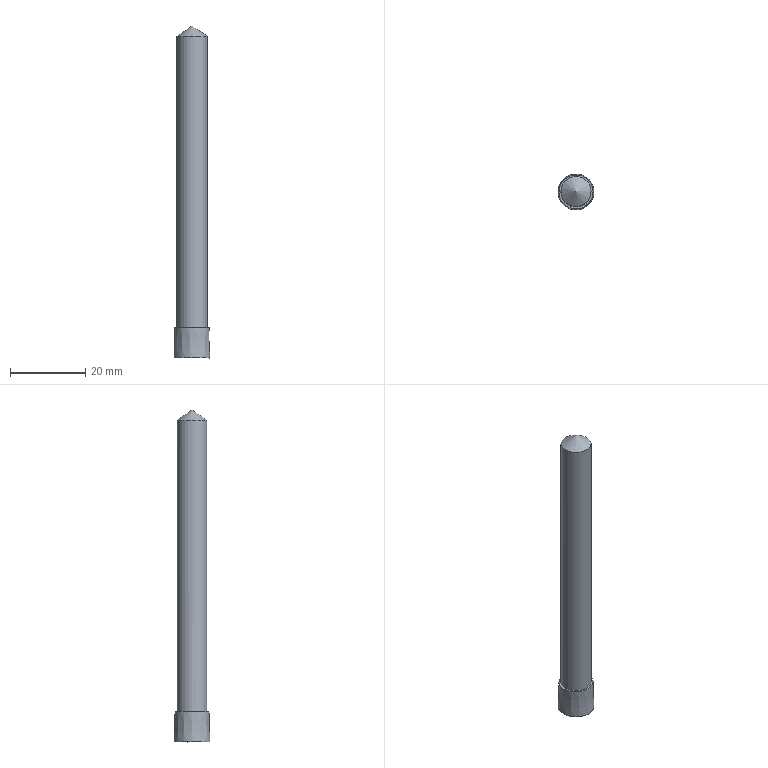Part | STEP file | 车灯-后视镜_id102_x_t | 1 solid | 5 faces | box 9.556 x 9.556 x 88.278 mm | volume 4490 mm3 | plane 2 | cone 2 | cylinder 1 | commonest cylinder face diameters 8 x1
STEP:
#1=CARTESIAN_POINT('',(-132.359,14.875,-27.286));
#2=VERTEX_POINT('',#1);
#3=CARTESIAN_POINT('',(-128.486,15.874,-27.286));
#4=DIRECTION('',(0.,0.,-1.));
#5=DIRECTION('',(-0.9683,-0.2497,0.));
#6=AXIS2_PLACEMENT_3D('',#3,#4,#5);
#7=CIRCLE('',#6,4.);
#8=EDGE_CURVE('',#2,#2,#7,.T.);
#9=ORIENTED_EDGE('',*,*,#8,.T.);
#10=EDGE_LOOP('',(#9));
#11=FACE_BOUND('',#10,.T.);
#12=CARTESIAN_POINT('',(-124.095,17.006,-27.286));
#13=VERTEX_POINT('',#12);
#14=CARTESIAN_POINT('',(-128.486,15.874,-27.286));
#15=DIRECTION('',(0.,0.,1.));
#16=DIRECTION('',(0.9683,0.2497,0.));
#17=AXIS2_PLACEMENT_3D('',#14,#15,#16);
#18=CIRCLE('',#17,4.535);
#19=EDGE_CURVE('',#13,#13,#18,.T.);
#20=ORIENTED_EDGE('',*,*,#19,.T.);
#21=EDGE_LOOP('',(#20));
#22=FACE_BOUND('',#21,.T.);
#23=CARTESIAN_POINT('',(-128.486,15.874,-27.286));
#24=DIRECTION('',(0.,0.,1.));
#25=DIRECTION('',(-0.9683,-0.2497,0.));
#26=AXIS2_PLACEMENT_3D('',#23,#24,#25);
#27=PLANE('',#26);
#28=ADVANCED_FACE('',(#11,#22),#27,.T.);
#29=CARTESIAN_POINT('',(-123.708,15.874,-35.286));
#30=VERTEX_POINT('',#29);
#31=CARTESIAN_POINT('',(-128.486,15.874,-35.286));
#32=DIRECTION('',(0.,0.,-1.));
#33=DIRECTION('',(1.,0.,0.));
#34=AXIS2_PLACEMENT_3D('',#31,#32,#33);
#35=CIRCLE('',#34,4.778);
#36=EDGE_CURVE('',#30,#30,#35,.T.);
#37=ORIENTED_EDGE('',*,*,#36,.F.);
#38=EDGE_LOOP('',(#37));
#39=FACE_BOUND('',#38,.T.);
#40=ORIENTED_EDGE('',*,*,#19,.F.);
#41=EDGE_LOOP('',(#40));
#42=FACE_BOUND('',#41,.T.);
#43=CARTESIAN_POINT('',(-128.486,15.874,-27.286));
#44=DIRECTION('',(0.,0.,-1.));
#45=DIRECTION('',(0.9683,0.2497,0.));
#46=AXIS2_PLACEMENT_3D('',#43,#44,#45);
#47=CONICAL_SURFACE('',#46,4.535,1.738);
#48=ADVANCED_FACE('',(#39,#42),#47,.T.);
#49=ORIENTED_EDGE('',*,*,#8,.F.);
#50=EDGE_LOOP('',(#49));
#51=FACE_BOUND('',#50,.T.);
#52=CARTESIAN_POINT('',(-132.486,15.874,50.294));
#53=VERTEX_POINT('',#52);
#54=CARTESIAN_POINT('',(-128.486,15.874,50.294));
#55=DIRECTION('',(0.,0.,1.));
#56=DIRECTION('',(-1.,0.,0.));
#57=AXIS2_PLACEMENT_3D('',#54,#55,#56);
#58=CIRCLE('',#57,4.);
#59=EDGE_CURVE('',#53,#53,#58,.T.);
#60=ORIENTED_EDGE('',*,*,#59,.F.);
#61=EDGE_LOOP('',(#60));
#62=FACE_BOUND('',#61,.T.);
#63=CARTESIAN_POINT('',(-128.486,15.874,-34.206));
#64=DIRECTION('',(0.,0.,1.));
#65=DIRECTION('',(-0.9683,-0.2497,0.));
#66=AXIS2_PLACEMENT_3D('',#63,#64,#65);
#67=CYLINDRICAL_SURFACE('',#66,4.);
#68=ADVANCED_FACE('',(#51,#62),#67,.T.);
#69=ORIENTED_EDGE('',*,*,#59,.T.);
#70=EDGE_LOOP('',(#69));
#71=FACE_BOUND('',#70,.T.);
#72=CARTESIAN_POINT('',(-128.486,15.874,52.992));
#73=VERTEX_POINT('',#72);
#74=VERTEX_LOOP('',#73);
#75=FACE_BOUND('',#74,.T.);
#76=CARTESIAN_POINT('',(-128.486,15.874,52.992));
#77=DIRECTION('',(0.,0.,-1.));
#78=DIRECTION('',(-0.9683,-0.2497,0.));
#79=AXIS2_PLACEMENT_3D('',#76,#77,#78);
#80=CONICAL_SURFACE('',#79,0.,56.);
#81=ADVANCED_FACE('',(#71,#75),#80,.T.);
#82=ORIENTED_EDGE('',*,*,#36,.T.);
#83=EDGE_LOOP('',(#82));
#84=FACE_OUTER_BOUND('',#83,.T.);
#85=CARTESIAN_POINT('',(-128.486,15.874,-35.286));
#86=DIRECTION('',(0.,0.,1.));
#87=DIRECTION('',(0.9683,0.2497,0.));
#88=AXIS2_PLACEMENT_3D('',#85,#86,#87);
#89=PLANE('',#88);
#90=ADVANCED_FACE('',(#84),#89,.F.);
#91=CLOSED_SHELL('',(#28,#48,#68,#81,#90));
#92=MANIFOLD_SOLID_BREP('',#91);
#93=(LENGTH_UNIT()NAMED_UNIT(*)SI_UNIT(.MILLI.,.METRE.));
#94=UNCERTAINTY_MEASURE_WITH_UNIT(LENGTH_MEASURE(0.00002),#93,'','');
#95=(NAMED_UNIT(*)PLANE_ANGLE_UNIT()SI_UNIT($,.RADIAN.));
#96=PLANE_ANGLE_MEASURE_WITH_UNIT(PLANE_ANGLE_MEASURE(0.01745),#95);
#97=DIMENSIONAL_EXPONENTS(0.,0.,0.,0.,0.,0.,0.);
#98=(CONVERSION_BASED_UNIT('DEGREE',#96)NAMED_UNIT(#97)PLANE_ANGLE_UNIT());
#99=(NAMED_UNIT(*)SI_UNIT($,.STERADIAN.)SOLID_ANGLE_UNIT());
#100=(GEOMETRIC_REPRESENTATION_CONTEXT(3)GLOBAL_UNCERTAINTY_ASSIGNED_CONTEXT((#94))GLOBAL_UNIT_ASSIGNED_CONTEXT((#93,#98,#99))REPRESENTATION_CONTEXT('',''));
#101=ADVANCED_BREP_SHAPE_REPRESENTATION('',(#92),#100);